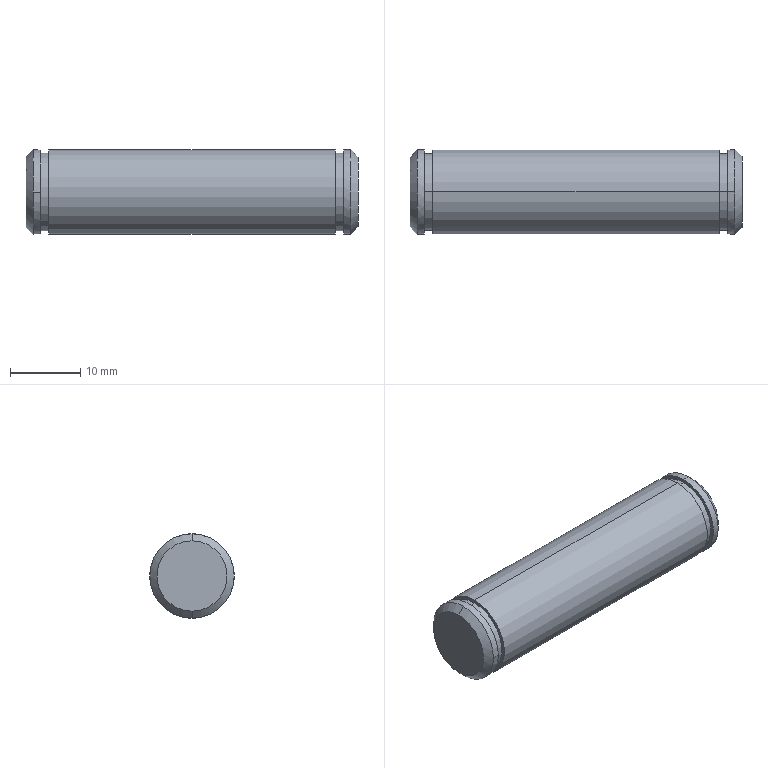Part | SolidWorks | features BaseBody 1 | 1 solid | 20 faces | box 47.2 x 12 x 12 mm | volume 5259 mm3 | cylinder 10 | plane 6 | cone 4 | commonest cylinder face diameters 12 x6 11 x4
STEP:
#1=CARTESIAN_POINT('',(-54.822,10.806,5.));
#2=VERTEX_POINT('',#1);
#3=CARTESIAN_POINT('',(-54.822,10.806,-5.));
#4=VERTEX_POINT('',#3);
#5=CARTESIAN_POINT('',(-54.822,10.806,0.));
#6=DIRECTION('',(-1.,0.,0.));
#7=DIRECTION('',(0.,0.,-1.));
#8=AXIS2_PLACEMENT_3D('',#5,#6,#7);
#9=CIRCLE('',#8,5.);
#10=EDGE_CURVE('',#2,#4,#9,.T.);
#11=ORIENTED_EDGE('',*,*,#10,.F.);
#12=CARTESIAN_POINT('',(-53.822,10.806,6.));
#13=VERTEX_POINT('',#12);
#14=CARTESIAN_POINT('',(-54.822,10.806,5.));
#15=DIRECTION('',(0.7071,0.,0.7071));
#16=VECTOR('',#15,1000.);
#17=LINE('',#14,#16);
#18=EDGE_CURVE('',#2,#13,#17,.T.);
#19=ORIENTED_EDGE('',*,*,#18,.T.);
#20=CARTESIAN_POINT('',(-53.822,16.806,0.));
#21=VERTEX_POINT('',#20);
#22=CARTESIAN_POINT('',(-53.822,10.806,0.));
#23=DIRECTION('',(1.,0.,0.));
#24=DIRECTION('',(0.,0.,-1.));
#25=AXIS2_PLACEMENT_3D('',#22,#23,#24);
#26=CIRCLE('',#25,6.);
#27=EDGE_CURVE('',#21,#13,#26,.T.);
#28=ORIENTED_EDGE('',*,*,#27,.F.);
#29=CARTESIAN_POINT('',(-53.822,10.806,-6.));
#30=VERTEX_POINT('',#29);
#31=CARTESIAN_POINT('',(-53.822,10.806,0.));
#32=DIRECTION('',(1.,0.,0.));
#33=DIRECTION('',(0.,0.,-1.));
#34=AXIS2_PLACEMENT_3D('',#31,#32,#33);
#35=CIRCLE('',#34,6.);
#36=EDGE_CURVE('',#30,#21,#35,.T.);
#37=ORIENTED_EDGE('',*,*,#36,.F.);
#38=CARTESIAN_POINT('',(-54.822,10.806,-5.));
#39=DIRECTION('',(0.7071,0.,-0.7071));
#40=VECTOR('',#39,1000.);
#41=LINE('',#38,#40);
#42=EDGE_CURVE('',#4,#30,#41,.T.);
#43=ORIENTED_EDGE('',*,*,#42,.F.);
#44=EDGE_LOOP('',(#11,#19,#28,#37,#43));
#45=FACE_OUTER_BOUND('',#44,.T.);
#46=CARTESIAN_POINT('',(-54.822,10.806,0.));
#47=DIRECTION('',(1.,0.,0.));
#48=DIRECTION('',(0.,0.,-1.));
#49=AXIS2_PLACEMENT_3D('',#46,#47,#48);
#50=CONICAL_SURFACE('',#49,5.,0.7854);
#51=ADVANCED_FACE('',(#45),#50,.T.);
#52=CARTESIAN_POINT('',(-52.822,16.806,0.));
#53=VERTEX_POINT('',#52);
#54=CARTESIAN_POINT('',(-52.822,4.806,0.));
#55=VERTEX_POINT('',#54);
#56=CARTESIAN_POINT('',(-52.822,10.806,0.));
#57=DIRECTION('',(1.,0.,0.));
#58=DIRECTION('',(0.,-1.,0.));
#59=AXIS2_PLACEMENT_3D('',#56,#57,#58);
#60=CIRCLE('',#59,6.);
#61=EDGE_CURVE('',#53,#55,#60,.T.);
#62=ORIENTED_EDGE('',*,*,#61,.F.);
#63=CARTESIAN_POINT('',(-52.822,16.806,0.));
#64=DIRECTION('',(-1.,0.,0.));
#65=VECTOR('',#64,1000.);
#66=LINE('',#63,#65);
#67=EDGE_CURVE('',#53,#21,#66,.T.);
#68=ORIENTED_EDGE('',*,*,#67,.T.);
#69=ORIENTED_EDGE('',*,*,#27,.T.);
#70=CARTESIAN_POINT('',(-53.822,4.806,0.));
#71=VERTEX_POINT('',#70);
#72=CARTESIAN_POINT('',(-53.822,10.806,0.));
#73=DIRECTION('',(1.,0.,0.));
#74=DIRECTION('',(0.,0.,-1.));
#75=AXIS2_PLACEMENT_3D('',#72,#73,#74);
#76=CIRCLE('',#75,6.);
#77=EDGE_CURVE('',#13,#71,#76,.T.);
#78=ORIENTED_EDGE('',*,*,#77,.T.);
#79=CARTESIAN_POINT('',(-52.822,4.806,0.));
#80=DIRECTION('',(-1.,0.,0.));
#81=VECTOR('',#80,1000.);
#82=LINE('',#79,#81);
#83=EDGE_CURVE('',#55,#71,#82,.T.);
#84=ORIENTED_EDGE('',*,*,#83,.F.);
#85=EDGE_LOOP('',(#62,#68,#69,#78,#84));
#86=FACE_OUTER_BOUND('',#85,.T.);
#87=CARTESIAN_POINT('',(-52.822,10.806,0.));
#88=DIRECTION('',(-1.,0.,0.));
#89=DIRECTION('',(0.,-1.,0.));
#90=AXIS2_PLACEMENT_3D('',#87,#88,#89);
#91=CYLINDRICAL_SURFACE('',#90,6.);
#92=ADVANCED_FACE('',(#86),#91,.T.);
#93=CARTESIAN_POINT('',(-51.622,10.806,-5.5));
#94=VERTEX_POINT('',#93);
#95=CARTESIAN_POINT('',(-51.622,10.806,5.5));
#96=VERTEX_POINT('',#95);
#97=CARTESIAN_POINT('',(-51.622,10.806,0.));
#98=DIRECTION('',(1.,0.,0.));
#99=DIRECTION('',(0.,0.,1.));
#100=AXIS2_PLACEMENT_3D('',#97,#98,#99);
#101=CIRCLE('',#100,5.5);
#102=EDGE_CURVE('',#94,#96,#101,.T.);
#103=ORIENTED_EDGE('',*,*,#102,.F.);
#104=CARTESIAN_POINT('',(-52.822,10.806,-5.5));
#105=VERTEX_POINT('',#104);
#106=CARTESIAN_POINT('',(-51.622,10.806,-5.5));
#107=DIRECTION('',(-1.,0.,0.));
#108=VECTOR('',#107,1000.);
#109=LINE('',#106,#108);
#110=EDGE_CURVE('',#94,#105,#109,.T.);
#111=ORIENTED_EDGE('',*,*,#110,.T.);
#112=CARTESIAN_POINT('',(-52.822,10.806,5.5));
#113=VERTEX_POINT('',#112);
#114=CARTESIAN_POINT('',(-52.822,10.806,0.));
#115=DIRECTION('',(1.,0.,0.));
#116=DIRECTION('',(0.,0.,1.));
#117=AXIS2_PLACEMENT_3D('',#114,#115,#116);
#118=CIRCLE('',#117,5.5);
#119=EDGE_CURVE('',#105,#113,#118,.T.);
#120=ORIENTED_EDGE('',*,*,#119,.T.);
#121=CARTESIAN_POINT('',(-51.622,10.806,5.5));
#122=DIRECTION('',(-1.,0.,0.));
#123=VECTOR('',#122,1000.);
#124=LINE('',#121,#123);
#125=EDGE_CURVE('',#96,#113,#124,.T.);
#126=ORIENTED_EDGE('',*,*,#125,.F.);
#127=EDGE_LOOP('',(#103,#111,#120,#126));
#128=FACE_OUTER_BOUND('',#127,.T.);
#129=CARTESIAN_POINT('',(-51.622,10.806,0.));
#130=DIRECTION('',(-1.,0.,0.));
#131=DIRECTION('',(0.,0.,1.));
#132=AXIS2_PLACEMENT_3D('',#129,#130,#131);
#133=CYLINDRICAL_SURFACE('',#132,5.5);
#134=ADVANCED_FACE('',(#128),#133,.T.);
#135=CARTESIAN_POINT('',(-10.822,10.806,-6.));
#136=VERTEX_POINT('',#135);
#137=CARTESIAN_POINT('',(-10.822,10.806,6.));
#138=VERTEX_POINT('',#137);
#139=CARTESIAN_POINT('',(-10.822,10.806,0.));
#140=DIRECTION('',(1.,0.,0.));
#141=DIRECTION('',(0.,0.,1.));
#142=AXIS2_PLACEMENT_3D('',#139,#140,#141);
#143=CIRCLE('',#142,6.);
#144=EDGE_CURVE('',#136,#138,#143,.T.);
#145=ORIENTED_EDGE('',*,*,#144,.F.);
#146=CARTESIAN_POINT('',(-51.622,10.806,-6.));
#147=VERTEX_POINT('',#146);
#148=CARTESIAN_POINT('',(-10.822,10.806,-6.));
#149=DIRECTION('',(-1.,0.,0.));
#150=VECTOR('',#149,1000.);
#151=LINE('',#148,#150);
#152=EDGE_CURVE('',#136,#147,#151,.T.);
#153=ORIENTED_EDGE('',*,*,#152,.T.);
#154=CARTESIAN_POINT('',(-51.622,10.806,6.));
#155=VERTEX_POINT('',#154);
#156=CARTESIAN_POINT('',(-51.622,10.806,0.));
#157=DIRECTION('',(1.,0.,0.));
#158=DIRECTION('',(0.,0.,1.));
#159=AXIS2_PLACEMENT_3D('',#156,#157,#158);
#160=CIRCLE('',#159,6.);
#161=EDGE_CURVE('',#147,#155,#160,.T.);
#162=ORIENTED_EDGE('',*,*,#161,.T.);
#163=CARTESIAN_POINT('',(-10.822,10.806,6.));
#164=DIRECTION('',(-1.,0.,0.));
#165=VECTOR('',#164,1000.);
#166=LINE('',#163,#165);
#167=EDGE_CURVE('',#138,#155,#166,.T.);
#168=ORIENTED_EDGE('',*,*,#167,.F.);
#169=EDGE_LOOP('',(#145,#153,#162,#168));
#170=FACE_OUTER_BOUND('',#169,.T.);
#171=CARTESIAN_POINT('',(-10.822,10.806,0.));
#172=DIRECTION('',(-1.,0.,0.));
#173=DIRECTION('',(0.,0.,1.));
#174=AXIS2_PLACEMENT_3D('',#171,#172,#173);
#175=CYLINDRICAL_SURFACE('',#174,6.);
#176=ADVANCED_FACE('',(#170),#175,.T.);
#177=CARTESIAN_POINT('',(-9.622,10.806,-5.5));
#178=VERTEX_POINT('',#177);
#179=CARTESIAN_POINT('',(-9.622,10.806,5.5));
#180=VERTEX_POINT('',#179);
#181=CARTESIAN_POINT('',(-9.622,10.806,0.));
#182=DIRECTION('',(1.,0.,0.));
#183=DIRECTION('',(0.,0.,1.));
#184=AXIS2_PLACEMENT_3D('',#181,#182,#183);
#185=CIRCLE('',#184,5.5);
#186=EDGE_CURVE('',#178,#180,#185,.T.);
#187=ORIENTED_EDGE('',*,*,#186,.F.);
#188=CARTESIAN_POINT('',(-10.822,10.806,-5.5));
#189=VERTEX_POINT('',#188);
#190=CARTESIAN_POINT('',(-9.622,10.806,-5.5));
#191=DIRECTION('',(-1.,0.,0.));
#192=VECTOR('',#191,1000.);
#193=LINE('',#190,#192);
#194=EDGE_CURVE('',#178,#189,#193,.T.);
#195=ORIENTED_EDGE('',*,*,#194,.T.);
#196=CARTESIAN_POINT('',(-10.822,10.806,5.5));
#197=VERTEX_POINT('',#196);
#198=CARTESIAN_POINT('',(-10.822,10.806,0.));
#199=DIRECTION('',(1.,0.,0.));
#200=DIRECTION('',(0.,0.,1.));
#201=AXIS2_PLACEMENT_3D('',#198,#199,#200);
#202=CIRCLE('',#201,5.5);
#203=EDGE_CURVE('',#189,#197,#202,.T.);
#204=ORIENTED_EDGE('',*,*,#203,.T.);
#205=CARTESIAN_POINT('',(-9.622,10.806,5.5));
#206=DIRECTION('',(-1.,0.,0.));
#207=VECTOR('',#206,1000.);
#208=LINE('',#205,#207);
#209=EDGE_CURVE('',#180,#197,#208,.T.);
#210=ORIENTED_EDGE('',*,*,#209,.F.);
#211=EDGE_LOOP('',(#187,#195,#204,#210));
#212=FACE_OUTER_BOUND('',#211,.T.);
#213=CARTESIAN_POINT('',(-9.622,10.806,0.));
#214=DIRECTION('',(-1.,0.,0.));
#215=DIRECTION('',(0.,0.,1.));
#216=AXIS2_PLACEMENT_3D('',#213,#214,#215);
#217=CYLINDRICAL_SURFACE('',#216,5.5);
#218=ADVANCED_FACE('',(#212),#217,.T.);
#219=CARTESIAN_POINT('',(-8.622,10.806,-6.));
#220=VERTEX_POINT('',#219);
#221=CARTESIAN_POINT('',(-8.622,16.806,0.));
#222=VERTEX_POINT('',#221);
#223=CARTESIAN_POINT('',(-8.622,10.806,0.));
#224=DIRECTION('',(1.,0.,0.));
#225=DIRECTION('',(0.,0.,1.));
#226=AXIS2_PLACEMENT_3D('',#223,#224,#225);
#227=CIRCLE('',#226,6.);
#228=EDGE_CURVE('',#220,#222,#227,.T.);
#229=ORIENTED_EDGE('',*,*,#228,.F.);
#230=CARTESIAN_POINT('',(-9.622,10.806,-6.));
#231=VERTEX_POINT('',#230);
#232=CARTESIAN_POINT('',(-8.622,10.806,-6.));
#233=DIRECTION('',(-1.,0.,0.));
#234=VECTOR('',#233,1000.);
#235=LINE('',#232,#234);
#236=EDGE_CURVE('',#220,#231,#235,.T.);
#237=ORIENTED_EDGE('',*,*,#236,.T.);
#238=CARTESIAN_POINT('',(-9.622,10.806,6.));
#239=VERTEX_POINT('',#238);
#240=CARTESIAN_POINT('',(-9.622,10.806,0.));
#241=DIRECTION('',(1.,0.,0.));
#242=DIRECTION('',(0.,0.,1.));
#243=AXIS2_PLACEMENT_3D('',#240,#241,#242);
#244=CIRCLE('',#243,6.);
#245=EDGE_CURVE('',#231,#239,#244,.T.);
#246=ORIENTED_EDGE('',*,*,#245,.T.);
#247=CARTESIAN_POINT('',(-8.622,10.806,6.));
#248=VERTEX_POINT('',#247);
#249=CARTESIAN_POINT('',(-8.622,10.806,6.));
#250=DIRECTION('',(-1.,0.,0.));
#251=VECTOR('',#250,1000.);
#252=LINE('',#249,#251);
#253=EDGE_CURVE('',#248,#239,#252,.T.);
#254=ORIENTED_EDGE('',*,*,#253,.F.);
#255=CARTESIAN_POINT('',(-8.622,10.806,0.));
#256=DIRECTION('',(1.,0.,0.));
#257=DIRECTION('',(0.,0.,1.));
#258=AXIS2_PLACEMENT_3D('',#255,#256,#257);
#259=CIRCLE('',#258,6.);
#260=EDGE_CURVE('',#222,#248,#259,.T.);
#261=ORIENTED_EDGE('',*,*,#260,.F.);
#262=EDGE_LOOP('',(#229,#237,#246,#254,#261));
#263=FACE_OUTER_BOUND('',#262,.T.);
#264=CARTESIAN_POINT('',(-8.622,10.806,0.));
#265=DIRECTION('',(-1.,0.,0.));
#266=DIRECTION('',(0.,0.,1.));
#267=AXIS2_PLACEMENT_3D('',#264,#265,#266);
#268=CYLINDRICAL_SURFACE('',#267,6.);
#269=ADVANCED_FACE('',(#263),#268,.T.);
#270=CARTESIAN_POINT('',(-7.622,15.806,0.));
#271=VERTEX_POINT('',#270);
#272=CARTESIAN_POINT('',(-7.622,5.806,0.));
#273=VERTEX_POINT('',#272);
#274=CARTESIAN_POINT('',(-7.622,10.806,0.));
#275=DIRECTION('',(1.,0.,0.));
#276=DIRECTION('',(0.,-1.,0.));
#277=AXIS2_PLACEMENT_3D('',#274,#275,#276);
#278=CIRCLE('',#277,5.);
#279=EDGE_CURVE('',#271,#273,#278,.T.);
#280=ORIENTED_EDGE('',*,*,#279,.F.);
#281=CARTESIAN_POINT('',(-7.622,15.806,0.));
#282=DIRECTION('',(-0.7071,0.7071,0.));
#283=VECTOR('',#282,1000.);
#284=LINE('',#281,#283);
#285=EDGE_CURVE('',#271,#222,#284,.T.);
#286=ORIENTED_EDGE('',*,*,#285,.T.);
#287=ORIENTED_EDGE('',*,*,#260,.T.);
#288=CARTESIAN_POINT('',(-8.622,4.806,0.));
#289=VERTEX_POINT('',#288);
#290=CARTESIAN_POINT('',(-8.622,10.806,0.));
#291=DIRECTION('',(1.,0.,0.));
#292=DIRECTION('',(0.,0.,1.));
#293=AXIS2_PLACEMENT_3D('',#290,#291,#292);
#294=CIRCLE('',#293,6.);
#295=EDGE_CURVE('',#248,#289,#294,.T.);
#296=ORIENTED_EDGE('',*,*,#295,.T.);
#297=CARTESIAN_POINT('',(-7.622,5.806,0.));
#298=DIRECTION('',(-0.7071,-0.7071,0.));
#299=VECTOR('',#298,1000.);
#300=LINE('',#297,#299);
#301=EDGE_CURVE('',#273,#289,#300,.T.);
#302=ORIENTED_EDGE('',*,*,#301,.F.);
#303=EDGE_LOOP('',(#280,#286,#287,#296,#302));
#304=FACE_OUTER_BOUND('',#303,.T.);
#305=CARTESIAN_POINT('',(-7.622,10.806,0.));
#306=DIRECTION('',(-1.,0.,0.));
#307=DIRECTION('',(0.,-1.,0.));
#308=AXIS2_PLACEMENT_3D('',#305,#306,#307);
#309=CONICAL_SURFACE('',#308,5.,0.7854);
#310=ADVANCED_FACE('',(#304),#309,.T.);
#311=ORIENTED_EDGE('',*,*,#18,.F.);
#312=CARTESIAN_POINT('',(-54.822,10.806,0.));
#313=DIRECTION('',(-1.,0.,0.));
#314=DIRECTION('',(0.,0.,-1.));
#315=AXIS2_PLACEMENT_3D('',#312,#313,#314);
#316=CIRCLE('',#315,5.);
#317=EDGE_CURVE('',#4,#2,#316,.T.);
#318=ORIENTED_EDGE('',*,*,#317,.F.);
#319=ORIENTED_EDGE('',*,*,#42,.T.);
#320=CARTESIAN_POINT('',(-53.822,10.806,0.));
#321=DIRECTION('',(1.,0.,0.));
#322=DIRECTION('',(0.,0.,-1.));
#323=AXIS2_PLACEMENT_3D('',#320,#321,#322);
#324=CIRCLE('',#323,6.);
#325=EDGE_CURVE('',#71,#30,#324,.T.);
#326=ORIENTED_EDGE('',*,*,#325,.F.);
#327=ORIENTED_EDGE('',*,*,#77,.F.);
#328=EDGE_LOOP('',(#311,#318,#319,#326,#327));
#329=FACE_OUTER_BOUND('',#328,.T.);
#330=CARTESIAN_POINT('',(-54.822,10.806,0.));
#331=DIRECTION('',(1.,0.,0.));
#332=DIRECTION('',(0.,0.,-1.));
#333=AXIS2_PLACEMENT_3D('',#330,#331,#332);
#334=CONICAL_SURFACE('',#333,5.,0.7854);
#335=ADVANCED_FACE('',(#329),#334,.T.);
#336=ORIENTED_EDGE('',*,*,#317,.T.);
#337=ORIENTED_EDGE('',*,*,#10,.T.);
#338=EDGE_LOOP('',(#336,#337));
#339=FACE_OUTER_BOUND('',#338,.T.);
#340=CARTESIAN_POINT('',(-54.822,5.746,5.06));
#341=DIRECTION('',(1.,0.,0.));
#342=DIRECTION('',(0.,0.,-1.));
#343=AXIS2_PLACEMENT_3D('',#340,#341,#342);
#344=PLANE('',#343);
#345=ADVANCED_FACE('',(#339),#344,.F.);
#346=ORIENTED_EDGE('',*,*,#67,.F.);
#347=CARTESIAN_POINT('',(-52.822,10.806,0.));
#348=DIRECTION('',(1.,0.,0.));
#349=DIRECTION('',(0.,-1.,0.));
#350=AXIS2_PLACEMENT_3D('',#347,#348,#349);
#351=CIRCLE('',#350,6.);
#352=EDGE_CURVE('',#55,#53,#351,.T.);
#353=ORIENTED_EDGE('',*,*,#352,.F.);
#354=ORIENTED_EDGE('',*,*,#83,.T.);
#355=ORIENTED_EDGE('',*,*,#325,.T.);
#356=ORIENTED_EDGE('',*,*,#36,.T.);
#357=EDGE_LOOP('',(#346,#353,#354,#355,#356));
#358=FACE_OUTER_BOUND('',#357,.T.);
#359=CARTESIAN_POINT('',(-52.822,10.806,0.));
#360=DIRECTION('',(-1.,0.,0.));
#361=DIRECTION('',(0.,-1.,0.));
#362=AXIS2_PLACEMENT_3D('',#359,#360,#361);
#363=CYLINDRICAL_SURFACE('',#362,6.);
#364=ADVANCED_FACE('',(#358),#363,.T.);
#365=CARTESIAN_POINT('',(-52.822,10.806,0.));
#366=DIRECTION('',(1.,0.,0.));
#367=DIRECTION('',(0.,0.,1.));
#368=AXIS2_PLACEMENT_3D('',#365,#366,#367);
#369=CIRCLE('',#368,5.5);
#370=EDGE_CURVE('',#113,#105,#369,.T.);
#371=ORIENTED_EDGE('',*,*,#370,.F.);
#372=ORIENTED_EDGE('',*,*,#119,.F.);
#373=EDGE_LOOP('',(#371,#372));
#374=FACE_BOUND('',#373,.T.);
#375=ORIENTED_EDGE('',*,*,#352,.T.);
#376=ORIENTED_EDGE('',*,*,#61,.T.);
#377=EDGE_LOOP('',(#375,#376));
#378=FACE_OUTER_BOUND('',#377,.T.);
#379=CARTESIAN_POINT('',(-52.822,4.734,-6.072));
#380=DIRECTION('',(-1.,0.,0.));
#381=DIRECTION('',(0.,0.,1.));
#382=AXIS2_PLACEMENT_3D('',#379,#380,#381);
#383=PLANE('',#382);
#384=ADVANCED_FACE('',(#374,#378),#383,.F.);
#385=ORIENTED_EDGE('',*,*,#110,.F.);
#386=CARTESIAN_POINT('',(-51.622,10.806,0.));
#387=DIRECTION('',(1.,0.,0.));
#388=DIRECTION('',(0.,0.,1.));
#389=AXIS2_PLACEMENT_3D('',#386,#387,#388);
#390=CIRCLE('',#389,5.5);
#391=EDGE_CURVE('',#96,#94,#390,.T.);
#392=ORIENTED_EDGE('',*,*,#391,.F.);
#393=ORIENTED_EDGE('',*,*,#125,.T.);
#394=ORIENTED_EDGE('',*,*,#370,.T.);
#395=EDGE_LOOP('',(#385,#392,#393,#394));
#396=FACE_OUTER_BOUND('',#395,.T.);
#397=CARTESIAN_POINT('',(-51.622,10.806,0.));
#398=DIRECTION('',(-1.,0.,0.));
#399=DIRECTION('',(0.,0.,1.));
#400=AXIS2_PLACEMENT_3D('',#397,#398,#399);
#401=CYLINDRICAL_SURFACE('',#400,5.5);
#402=ADVANCED_FACE('',(#396),#401,.T.);
#403=ORIENTED_EDGE('',*,*,#391,.T.);
#404=ORIENTED_EDGE('',*,*,#102,.T.);
#405=EDGE_LOOP('',(#403,#404));
#406=FACE_BOUND('',#405,.T.);
#407=CARTESIAN_POINT('',(-51.622,10.806,0.));
#408=DIRECTION('',(1.,0.,0.));
#409=DIRECTION('',(0.,0.,1.));
#410=AXIS2_PLACEMENT_3D('',#407,#408,#409);
#411=CIRCLE('',#410,6.);
#412=EDGE_CURVE('',#155,#147,#411,.T.);
#413=ORIENTED_EDGE('',*,*,#412,.F.);
#414=ORIENTED_EDGE('',*,*,#161,.F.);
#415=EDGE_LOOP('',(#413,#414));
#416=FACE_OUTER_BOUND('',#415,.T.);
#417=CARTESIAN_POINT('',(-51.622,4.734,6.072));
#418=DIRECTION('',(1.,0.,0.));
#419=DIRECTION('',(0.,0.,-1.));
#420=AXIS2_PLACEMENT_3D('',#417,#418,#419);
#421=PLANE('',#420);
#422=ADVANCED_FACE('',(#406,#416),#421,.F.);
#423=ORIENTED_EDGE('',*,*,#152,.F.);
#424=CARTESIAN_POINT('',(-10.822,10.806,0.));
#425=DIRECTION('',(1.,0.,0.));
#426=DIRECTION('',(0.,0.,1.));
#427=AXIS2_PLACEMENT_3D('',#424,#425,#426);
#428=CIRCLE('',#427,6.);
#429=EDGE_CURVE('',#138,#136,#428,.T.);
#430=ORIENTED_EDGE('',*,*,#429,.F.);
#431=ORIENTED_EDGE('',*,*,#167,.T.);
#432=ORIENTED_EDGE('',*,*,#412,.T.);
#433=EDGE_LOOP('',(#423,#430,#431,#432));
#434=FACE_OUTER_BOUND('',#433,.T.);
#435=CARTESIAN_POINT('',(-10.822,10.806,0.));
#436=DIRECTION('',(-1.,0.,0.));
#437=DIRECTION('',(0.,0.,1.));
#438=AXIS2_PLACEMENT_3D('',#435,#436,#437);
#439=CYLINDRICAL_SURFACE('',#438,6.);
#440=ADVANCED_FACE('',(#434),#439,.T.);
#441=CARTESIAN_POINT('',(-10.822,10.806,0.));
#442=DIRECTION('',(1.,0.,0.));
#443=DIRECTION('',(0.,0.,1.));
#444=AXIS2_PLACEMENT_3D('',#441,#442,#443);
#445=CIRCLE('',#444,5.5);
#446=EDGE_CURVE('',#197,#189,#445,.T.);
#447=ORIENTED_EDGE('',*,*,#446,.F.);
#448=ORIENTED_EDGE('',*,*,#203,.F.);
#449=EDGE_LOOP('',(#447,#448));
#450=FACE_BOUND('',#449,.T.);
#451=ORIENTED_EDGE('',*,*,#429,.T.);
#452=ORIENTED_EDGE('',*,*,#144,.T.);
#453=EDGE_LOOP('',(#451,#452));
#454=FACE_OUTER_BOUND('',#453,.T.);
#455=CARTESIAN_POINT('',(-10.822,4.734,-6.072));
#456=DIRECTION('',(-1.,0.,0.));
#457=DIRECTION('',(0.,0.,1.));
#458=AXIS2_PLACEMENT_3D('',#455,#456,#457);
#459=PLANE('',#458);
#460=ADVANCED_FACE('',(#450,#454),#459,.F.);
#461=ORIENTED_EDGE('',*,*,#194,.F.);
#462=CARTESIAN_POINT('',(-9.622,10.806,0.));
#463=DIRECTION('',(1.,0.,0.));
#464=DIRECTION('',(0.,0.,1.));
#465=AXIS2_PLACEMENT_3D('',#462,#463,#464);
#466=CIRCLE('',#465,5.5);
#467=EDGE_CURVE('',#180,#178,#466,.T.);
#468=ORIENTED_EDGE('',*,*,#467,.F.);
#469=ORIENTED_EDGE('',*,*,#209,.T.);
#470=ORIENTED_EDGE('',*,*,#446,.T.);
#471=EDGE_LOOP('',(#461,#468,#469,#470));
#472=FACE_OUTER_BOUND('',#471,.T.);
#473=CARTESIAN_POINT('',(-9.622,10.806,0.));
#474=DIRECTION('',(-1.,0.,0.));
#475=DIRECTION('',(0.,0.,1.));
#476=AXIS2_PLACEMENT_3D('',#473,#474,#475);
#477=CYLINDRICAL_SURFACE('',#476,5.5);
#478=ADVANCED_FACE('',(#472),#477,.T.);
#479=ORIENTED_EDGE('',*,*,#467,.T.);
#480=ORIENTED_EDGE('',*,*,#186,.T.);
#481=EDGE_LOOP('',(#479,#480));
#482=FACE_BOUND('',#481,.T.);
#483=CARTESIAN_POINT('',(-9.622,10.806,0.));
#484=DIRECTION('',(1.,0.,0.));
#485=DIRECTION('',(0.,0.,1.));
#486=AXIS2_PLACEMENT_3D('',#483,#484,#485);
#487=CIRCLE('',#486,6.);
#488=EDGE_CURVE('',#239,#231,#487,.T.);
#489=ORIENTED_EDGE('',*,*,#488,.F.);
#490=ORIENTED_EDGE('',*,*,#245,.F.);
#491=EDGE_LOOP('',(#489,#490));
#492=FACE_OUTER_BOUND('',#491,.T.);
#493=CARTESIAN_POINT('',(-9.622,4.734,6.072));
#494=DIRECTION('',(1.,0.,0.));
#495=DIRECTION('',(0.,0.,-1.));
#496=AXIS2_PLACEMENT_3D('',#493,#494,#495);
#497=PLANE('',#496);
#498=ADVANCED_FACE('',(#482,#492),#497,.F.);
#499=ORIENTED_EDGE('',*,*,#236,.F.);
#500=CARTESIAN_POINT('',(-8.622,10.806,0.));
#501=DIRECTION('',(1.,0.,0.));
#502=DIRECTION('',(0.,0.,1.));
#503=AXIS2_PLACEMENT_3D('',#500,#501,#502);
#504=CIRCLE('',#503,6.);
#505=EDGE_CURVE('',#289,#220,#504,.T.);
#506=ORIENTED_EDGE('',*,*,#505,.F.);
#507=ORIENTED_EDGE('',*,*,#295,.F.);
#508=ORIENTED_EDGE('',*,*,#253,.T.);
#509=ORIENTED_EDGE('',*,*,#488,.T.);
#510=EDGE_LOOP('',(#499,#506,#507,#508,#509));
#511=FACE_OUTER_BOUND('',#510,.T.);
#512=CARTESIAN_POINT('',(-8.622,10.806,0.));
#513=DIRECTION('',(-1.,0.,0.));
#514=DIRECTION('',(0.,0.,1.));
#515=AXIS2_PLACEMENT_3D('',#512,#513,#514);
#516=CYLINDRICAL_SURFACE('',#515,6.);
#517=ADVANCED_FACE('',(#511),#516,.T.);
#518=ORIENTED_EDGE('',*,*,#285,.F.);
#519=CARTESIAN_POINT('',(-7.622,10.806,0.));
#520=DIRECTION('',(1.,0.,0.));
#521=DIRECTION('',(0.,-1.,0.));
#522=AXIS2_PLACEMENT_3D('',#519,#520,#521);
#523=CIRCLE('',#522,5.);
#524=EDGE_CURVE('',#273,#271,#523,.T.);
#525=ORIENTED_EDGE('',*,*,#524,.F.);
#526=ORIENTED_EDGE('',*,*,#301,.T.);
#527=ORIENTED_EDGE('',*,*,#505,.T.);
#528=ORIENTED_EDGE('',*,*,#228,.T.);
#529=EDGE_LOOP('',(#518,#525,#526,#527,#528));
#530=FACE_OUTER_BOUND('',#529,.T.);
#531=CARTESIAN_POINT('',(-7.622,10.806,0.));
#532=DIRECTION('',(-1.,0.,0.));
#533=DIRECTION('',(0.,-1.,0.));
#534=AXIS2_PLACEMENT_3D('',#531,#532,#533);
#535=CONICAL_SURFACE('',#534,5.,0.7854);
#536=ADVANCED_FACE('',(#530),#535,.T.);
#537=ORIENTED_EDGE('',*,*,#524,.T.);
#538=ORIENTED_EDGE('',*,*,#279,.T.);
#539=EDGE_LOOP('',(#537,#538));
#540=FACE_OUTER_BOUND('',#539,.T.);
#541=CARTESIAN_POINT('',(-7.622,5.746,-5.06));
#542=DIRECTION('',(-1.,0.,0.));
#543=DIRECTION('',(0.,0.,1.));
#544=AXIS2_PLACEMENT_3D('',#541,#542,#543);
#545=PLANE('',#544);
#546=ADVANCED_FACE('',(#540),#545,.F.);
#547=CLOSED_SHELL('',(#51,#92,#134,#176,#218,#269,#310,#335,#345,#364,#384,#402,#422,#440,#460,#478,#498,#517,#536,#546));
#548=MANIFOLD_SOLID_BREP('',#547);
#549=CARTESIAN_POINT('',(0.,0.,0.));
#550=DIRECTION('',(0.,0.,1.));
#551=DIRECTION('',(1.,0.,0.));
#552=AXIS2_PLACEMENT_3D('',#549,#550,#551);
#553=(LENGTH_UNIT()NAMED_UNIT(*)SI_UNIT(.MILLI.,.METRE.));
#554=UNCERTAINTY_MEASURE_WITH_UNIT(LENGTH_MEASURE(0.00001),#553,'','');
#555=(NAMED_UNIT(*)PLANE_ANGLE_UNIT()SI_UNIT($,.RADIAN.));
#556=(NAMED_UNIT(*)SI_UNIT($,.STERADIAN.)SOLID_ANGLE_UNIT());
#557=(GEOMETRIC_REPRESENTATION_CONTEXT(3)GLOBAL_UNCERTAINTY_ASSIGNED_CONTEXT((#554))GLOBAL_UNIT_ASSIGNED_CONTEXT((#553,#555,#556))REPRESENTATION_CONTEXT('',''));
#558=ADVANCED_BREP_SHAPE_REPRESENTATION('',(#548,#552),#557);